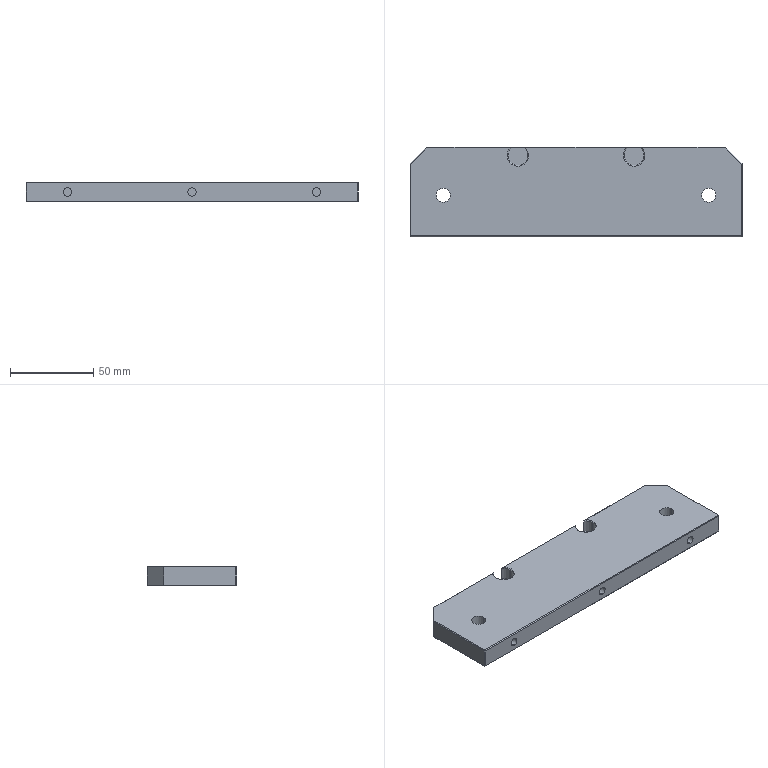Part | STEP file | Rotor mismatch mid plate | 1 solid | 64 faces | box 200 x 54 x 12 mm | volume 123822 mm3 | plane 41 | cylinder 18 | cone 5 | commonest cylinder face diameters 12 x8 5 x6 8.5 x4